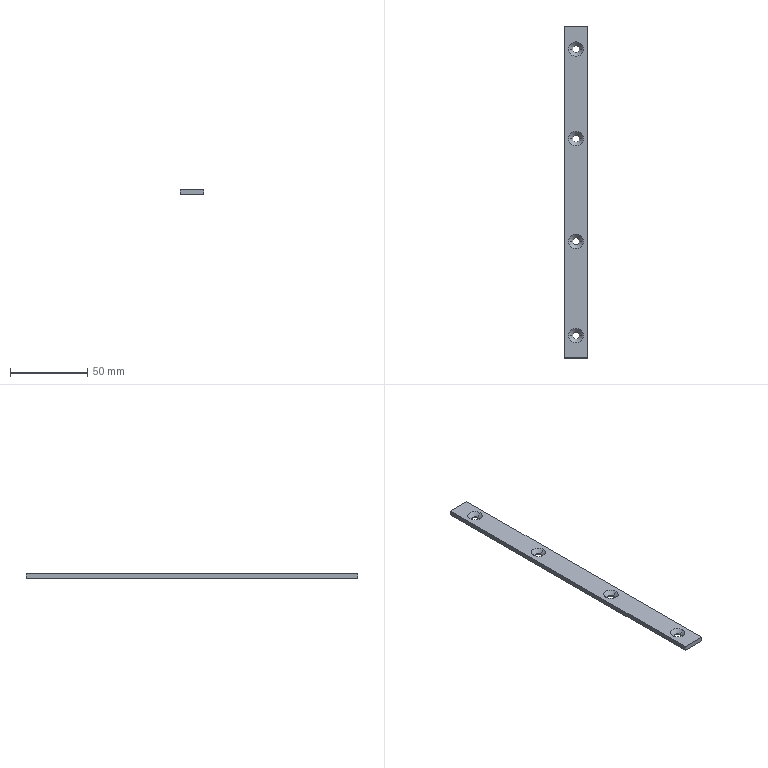Part | NX | features BREP 1 | 1 solid | 22 faces | box 15 x 215 x 3 mm | volume 9253 mm3 | cone 8 | cylinder 8 | plane 6 | commonest cylinder face diameters 4.5 x8
STEP:
#1=CARTESIAN_POINT('',(-4.7,-93.,3.));
#2=VERTEX_POINT('',#1);
#3=CARTESIAN_POINT('',(-2.25,-93.,0.55));
#4=VERTEX_POINT('',#3);
#5=CARTESIAN_POINT('',(-4.7,-93.,3.));
#6=DIRECTION('',(-0.7071,0.,0.7071));
#7=VECTOR('',#6,1000.);
#8=LINE('',#5,#7);
#9=EDGE_CURVE('',#2,#4,#8,.F.);
#10=ORIENTED_EDGE('',*,*,#9,.T.);
#11=CARTESIAN_POINT('',(2.25,-93.,0.55));
#12=VERTEX_POINT('',#11);
#13=CARTESIAN_POINT('',(0.,-93.,0.55));
#14=DIRECTION('',(0.,0.,1.));
#15=DIRECTION('',(1.,0.,0.));
#16=AXIS2_PLACEMENT_3D('',#13,#14,#15);
#17=CIRCLE('',#16,2.25);
#18=EDGE_CURVE('',#12,#4,#17,.T.);
#19=ORIENTED_EDGE('',*,*,#18,.F.);
#20=CARTESIAN_POINT('',(4.7,-93.,3.));
#21=VERTEX_POINT('',#20);
#22=CARTESIAN_POINT('',(4.7,-93.,3.));
#23=DIRECTION('',(0.7071,0.,0.7071));
#24=VECTOR('',#23,1000.);
#25=LINE('',#22,#24);
#26=EDGE_CURVE('',#21,#12,#25,.F.);
#27=ORIENTED_EDGE('',*,*,#26,.F.);
#28=CARTESIAN_POINT('',(0.,-93.,3.));
#29=DIRECTION('',(0.,0.,1.));
#30=DIRECTION('',(1.,0.,0.));
#31=AXIS2_PLACEMENT_3D('',#28,#29,#30);
#32=CIRCLE('',#31,4.7);
#33=EDGE_CURVE('',#21,#2,#32,.T.);
#34=ORIENTED_EDGE('',*,*,#33,.T.);
#35=EDGE_LOOP('',(#10,#19,#27,#34));
#36=FACE_BOUND('',#35,.T.);
#37=CARTESIAN_POINT('',(0.,-93.,3.));
#38=DIRECTION('',(0.,0.,1.));
#39=DIRECTION('',(1.,0.,0.));
#40=AXIS2_PLACEMENT_3D('',#37,#38,#39);
#41=CONICAL_SURFACE('',#40,4.7,0.7854);
#42=ADVANCED_FACE('',(#36),#41,.F.);
#43=CARTESIAN_POINT('',(-2.25,-93.,0.));
#44=VERTEX_POINT('',#43);
#45=CARTESIAN_POINT('',(-2.25,-93.,3.));
#46=DIRECTION('',(0.,0.,1.));
#47=VECTOR('',#46,1000.);
#48=LINE('',#45,#47);
#49=EDGE_CURVE('',#4,#44,#48,.F.);
#50=ORIENTED_EDGE('',*,*,#49,.T.);
#51=CARTESIAN_POINT('',(2.25,-93.,0.));
#52=VERTEX_POINT('',#51);
#53=CARTESIAN_POINT('',(0.,-93.,0.));
#54=DIRECTION('',(0.,0.,-1.));
#55=DIRECTION('',(-1.,0.,0.));
#56=AXIS2_PLACEMENT_3D('',#53,#54,#55);
#57=CIRCLE('',#56,2.25);
#58=EDGE_CURVE('',#44,#52,#57,.T.);
#59=ORIENTED_EDGE('',*,*,#58,.T.);
#60=CARTESIAN_POINT('',(2.25,-93.,3.));
#61=DIRECTION('',(0.,0.,1.));
#62=VECTOR('',#61,1000.);
#63=LINE('',#60,#62);
#64=EDGE_CURVE('',#12,#52,#63,.F.);
#65=ORIENTED_EDGE('',*,*,#64,.F.);
#66=ORIENTED_EDGE('',*,*,#18,.T.);
#67=EDGE_LOOP('',(#50,#59,#65,#66));
#68=FACE_BOUND('',#67,.T.);
#69=CARTESIAN_POINT('',(0.,-93.,3.));
#70=DIRECTION('',(0.,0.,1.));
#71=DIRECTION('',(1.,0.,0.));
#72=AXIS2_PLACEMENT_3D('',#69,#70,#71);
#73=CYLINDRICAL_SURFACE('',#72,2.25);
#74=ADVANCED_FACE('',(#68),#73,.F.);
#75=CARTESIAN_POINT('',(-4.7,-32.,3.));
#76=VERTEX_POINT('',#75);
#77=CARTESIAN_POINT('',(-2.25,-32.,0.55));
#78=VERTEX_POINT('',#77);
#79=CARTESIAN_POINT('',(-4.7,-32.,3.));
#80=DIRECTION('',(-0.7071,0.,0.7071));
#81=VECTOR('',#80,1000.);
#82=LINE('',#79,#81);
#83=EDGE_CURVE('',#76,#78,#82,.F.);
#84=ORIENTED_EDGE('',*,*,#83,.T.);
#85=CARTESIAN_POINT('',(2.25,-32.,0.55));
#86=VERTEX_POINT('',#85);
#87=CARTESIAN_POINT('',(0.,-32.,0.55));
#88=DIRECTION('',(0.,0.,1.));
#89=DIRECTION('',(1.,0.,0.));
#90=AXIS2_PLACEMENT_3D('',#87,#88,#89);
#91=CIRCLE('',#90,2.25);
#92=EDGE_CURVE('',#86,#78,#91,.T.);
#93=ORIENTED_EDGE('',*,*,#92,.F.);
#94=CARTESIAN_POINT('',(4.7,-32.,3.));
#95=VERTEX_POINT('',#94);
#96=CARTESIAN_POINT('',(4.7,-32.,3.));
#97=DIRECTION('',(0.7071,0.,0.7071));
#98=VECTOR('',#97,1000.);
#99=LINE('',#96,#98);
#100=EDGE_CURVE('',#95,#86,#99,.F.);
#101=ORIENTED_EDGE('',*,*,#100,.F.);
#102=CARTESIAN_POINT('',(0.,-32.,3.));
#103=DIRECTION('',(0.,0.,1.));
#104=DIRECTION('',(1.,0.,0.));
#105=AXIS2_PLACEMENT_3D('',#102,#103,#104);
#106=CIRCLE('',#105,4.7);
#107=EDGE_CURVE('',#95,#76,#106,.T.);
#108=ORIENTED_EDGE('',*,*,#107,.T.);
#109=EDGE_LOOP('',(#84,#93,#101,#108));
#110=FACE_BOUND('',#109,.T.);
#111=CARTESIAN_POINT('',(0.,-32.,3.));
#112=DIRECTION('',(0.,0.,1.));
#113=DIRECTION('',(1.,0.,0.));
#114=AXIS2_PLACEMENT_3D('',#111,#112,#113);
#115=CONICAL_SURFACE('',#114,4.7,0.7854);
#116=ADVANCED_FACE('',(#110),#115,.F.);
#117=CARTESIAN_POINT('',(-2.25,-32.,0.));
#118=VERTEX_POINT('',#117);
#119=CARTESIAN_POINT('',(-2.25,-32.,3.));
#120=DIRECTION('',(0.,0.,1.));
#121=VECTOR('',#120,1000.);
#122=LINE('',#119,#121);
#123=EDGE_CURVE('',#78,#118,#122,.F.);
#124=ORIENTED_EDGE('',*,*,#123,.T.);
#125=CARTESIAN_POINT('',(2.25,-32.,0.));
#126=VERTEX_POINT('',#125);
#127=CARTESIAN_POINT('',(0.,-32.,0.));
#128=DIRECTION('',(0.,0.,-1.));
#129=DIRECTION('',(-1.,0.,0.));
#130=AXIS2_PLACEMENT_3D('',#127,#128,#129);
#131=CIRCLE('',#130,2.25);
#132=EDGE_CURVE('',#118,#126,#131,.T.);
#133=ORIENTED_EDGE('',*,*,#132,.T.);
#134=CARTESIAN_POINT('',(2.25,-32.,3.));
#135=DIRECTION('',(0.,0.,1.));
#136=VECTOR('',#135,1000.);
#137=LINE('',#134,#136);
#138=EDGE_CURVE('',#86,#126,#137,.F.);
#139=ORIENTED_EDGE('',*,*,#138,.F.);
#140=ORIENTED_EDGE('',*,*,#92,.T.);
#141=EDGE_LOOP('',(#124,#133,#139,#140));
#142=FACE_BOUND('',#141,.T.);
#143=CARTESIAN_POINT('',(0.,-32.,3.));
#144=DIRECTION('',(0.,0.,1.));
#145=DIRECTION('',(1.,0.,0.));
#146=AXIS2_PLACEMENT_3D('',#143,#144,#145);
#147=CYLINDRICAL_SURFACE('',#146,2.25);
#148=ADVANCED_FACE('',(#142),#147,.F.);
#149=CARTESIAN_POINT('',(-4.7,34.5,3.));
#150=VERTEX_POINT('',#149);
#151=CARTESIAN_POINT('',(-2.25,34.5,0.55));
#152=VERTEX_POINT('',#151);
#153=CARTESIAN_POINT('',(-4.7,34.5,3.));
#154=DIRECTION('',(-0.7071,0.,0.7071));
#155=VECTOR('',#154,1000.);
#156=LINE('',#153,#155);
#157=EDGE_CURVE('',#150,#152,#156,.F.);
#158=ORIENTED_EDGE('',*,*,#157,.T.);
#159=CARTESIAN_POINT('',(2.25,34.5,0.55));
#160=VERTEX_POINT('',#159);
#161=CARTESIAN_POINT('',(0.,34.5,0.55));
#162=DIRECTION('',(0.,0.,1.));
#163=DIRECTION('',(1.,0.,0.));
#164=AXIS2_PLACEMENT_3D('',#161,#162,#163);
#165=CIRCLE('',#164,2.25);
#166=EDGE_CURVE('',#160,#152,#165,.T.);
#167=ORIENTED_EDGE('',*,*,#166,.F.);
#168=CARTESIAN_POINT('',(4.7,34.5,3.));
#169=VERTEX_POINT('',#168);
#170=CARTESIAN_POINT('',(4.7,34.5,3.));
#171=DIRECTION('',(0.7071,0.,0.7071));
#172=VECTOR('',#171,1000.);
#173=LINE('',#170,#172);
#174=EDGE_CURVE('',#169,#160,#173,.F.);
#175=ORIENTED_EDGE('',*,*,#174,.F.);
#176=CARTESIAN_POINT('',(0.,34.5,3.));
#177=DIRECTION('',(0.,0.,1.));
#178=DIRECTION('',(1.,0.,0.));
#179=AXIS2_PLACEMENT_3D('',#176,#177,#178);
#180=CIRCLE('',#179,4.7);
#181=EDGE_CURVE('',#169,#150,#180,.T.);
#182=ORIENTED_EDGE('',*,*,#181,.T.);
#183=EDGE_LOOP('',(#158,#167,#175,#182));
#184=FACE_BOUND('',#183,.T.);
#185=CARTESIAN_POINT('',(0.,34.5,3.));
#186=DIRECTION('',(0.,0.,1.));
#187=DIRECTION('',(1.,0.,0.));
#188=AXIS2_PLACEMENT_3D('',#185,#186,#187);
#189=CONICAL_SURFACE('',#188,4.7,0.7854);
#190=ADVANCED_FACE('',(#184),#189,.F.);
#191=CARTESIAN_POINT('',(-2.25,34.5,0.));
#192=VERTEX_POINT('',#191);
#193=CARTESIAN_POINT('',(-2.25,34.5,3.));
#194=DIRECTION('',(0.,0.,1.));
#195=VECTOR('',#194,1000.);
#196=LINE('',#193,#195);
#197=EDGE_CURVE('',#152,#192,#196,.F.);
#198=ORIENTED_EDGE('',*,*,#197,.T.);
#199=CARTESIAN_POINT('',(2.25,34.5,0.));
#200=VERTEX_POINT('',#199);
#201=CARTESIAN_POINT('',(0.,34.5,0.));
#202=DIRECTION('',(0.,0.,-1.));
#203=DIRECTION('',(-1.,0.,0.));
#204=AXIS2_PLACEMENT_3D('',#201,#202,#203);
#205=CIRCLE('',#204,2.25);
#206=EDGE_CURVE('',#192,#200,#205,.T.);
#207=ORIENTED_EDGE('',*,*,#206,.T.);
#208=CARTESIAN_POINT('',(2.25,34.5,3.));
#209=DIRECTION('',(0.,0.,1.));
#210=VECTOR('',#209,1000.);
#211=LINE('',#208,#210);
#212=EDGE_CURVE('',#160,#200,#211,.F.);
#213=ORIENTED_EDGE('',*,*,#212,.F.);
#214=ORIENTED_EDGE('',*,*,#166,.T.);
#215=EDGE_LOOP('',(#198,#207,#213,#214));
#216=FACE_BOUND('',#215,.T.);
#217=CARTESIAN_POINT('',(0.,34.5,3.));
#218=DIRECTION('',(0.,0.,1.));
#219=DIRECTION('',(1.,0.,0.));
#220=AXIS2_PLACEMENT_3D('',#217,#218,#219);
#221=CYLINDRICAL_SURFACE('',#220,2.25);
#222=ADVANCED_FACE('',(#216),#221,.F.);
#223=CARTESIAN_POINT('',(-4.7,92.5,3.));
#224=VERTEX_POINT('',#223);
#225=CARTESIAN_POINT('',(-2.25,92.5,0.55));
#226=VERTEX_POINT('',#225);
#227=CARTESIAN_POINT('',(-4.7,92.5,3.));
#228=DIRECTION('',(-0.7071,0.,0.7071));
#229=VECTOR('',#228,1000.);
#230=LINE('',#227,#229);
#231=EDGE_CURVE('',#224,#226,#230,.F.);
#232=ORIENTED_EDGE('',*,*,#231,.T.);
#233=CARTESIAN_POINT('',(2.25,92.5,0.55));
#234=VERTEX_POINT('',#233);
#235=CARTESIAN_POINT('',(0.,92.5,0.55));
#236=DIRECTION('',(0.,0.,1.));
#237=DIRECTION('',(1.,0.,0.));
#238=AXIS2_PLACEMENT_3D('',#235,#236,#237);
#239=CIRCLE('',#238,2.25);
#240=EDGE_CURVE('',#234,#226,#239,.T.);
#241=ORIENTED_EDGE('',*,*,#240,.F.);
#242=CARTESIAN_POINT('',(4.7,92.5,3.));
#243=VERTEX_POINT('',#242);
#244=CARTESIAN_POINT('',(4.7,92.5,3.));
#245=DIRECTION('',(0.7071,0.,0.7071));
#246=VECTOR('',#245,1000.);
#247=LINE('',#244,#246);
#248=EDGE_CURVE('',#243,#234,#247,.F.);
#249=ORIENTED_EDGE('',*,*,#248,.F.);
#250=CARTESIAN_POINT('',(0.,92.5,3.));
#251=DIRECTION('',(0.,0.,1.));
#252=DIRECTION('',(1.,0.,0.));
#253=AXIS2_PLACEMENT_3D('',#250,#251,#252);
#254=CIRCLE('',#253,4.7);
#255=EDGE_CURVE('',#243,#224,#254,.T.);
#256=ORIENTED_EDGE('',*,*,#255,.T.);
#257=EDGE_LOOP('',(#232,#241,#249,#256));
#258=FACE_BOUND('',#257,.T.);
#259=CARTESIAN_POINT('',(0.,92.5,3.));
#260=DIRECTION('',(0.,0.,1.));
#261=DIRECTION('',(1.,0.,0.));
#262=AXIS2_PLACEMENT_3D('',#259,#260,#261);
#263=CONICAL_SURFACE('',#262,4.7,0.7854);
#264=ADVANCED_FACE('',(#258),#263,.F.);
#265=CARTESIAN_POINT('',(-2.25,92.5,0.));
#266=VERTEX_POINT('',#265);
#267=CARTESIAN_POINT('',(-2.25,92.5,3.));
#268=DIRECTION('',(0.,0.,1.));
#269=VECTOR('',#268,1000.);
#270=LINE('',#267,#269);
#271=EDGE_CURVE('',#226,#266,#270,.F.);
#272=ORIENTED_EDGE('',*,*,#271,.T.);
#273=CARTESIAN_POINT('',(2.25,92.5,0.));
#274=VERTEX_POINT('',#273);
#275=CARTESIAN_POINT('',(0.,92.5,0.));
#276=DIRECTION('',(0.,0.,-1.));
#277=DIRECTION('',(-1.,0.,0.));
#278=AXIS2_PLACEMENT_3D('',#275,#276,#277);
#279=CIRCLE('',#278,2.25);
#280=EDGE_CURVE('',#266,#274,#279,.T.);
#281=ORIENTED_EDGE('',*,*,#280,.T.);
#282=CARTESIAN_POINT('',(2.25,92.5,3.));
#283=DIRECTION('',(0.,0.,1.));
#284=VECTOR('',#283,1000.);
#285=LINE('',#282,#284);
#286=EDGE_CURVE('',#234,#274,#285,.F.);
#287=ORIENTED_EDGE('',*,*,#286,.F.);
#288=ORIENTED_EDGE('',*,*,#240,.T.);
#289=EDGE_LOOP('',(#272,#281,#287,#288));
#290=FACE_BOUND('',#289,.T.);
#291=CARTESIAN_POINT('',(0.,92.5,3.));
#292=DIRECTION('',(0.,0.,1.));
#293=DIRECTION('',(1.,0.,0.));
#294=AXIS2_PLACEMENT_3D('',#291,#292,#293);
#295=CYLINDRICAL_SURFACE('',#294,2.25);
#296=ADVANCED_FACE('',(#290),#295,.F.);
#297=CARTESIAN_POINT('',(7.5,-107.5,0.));
#298=VERTEX_POINT('',#297);
#299=CARTESIAN_POINT('',(7.5,107.5,0.));
#300=VERTEX_POINT('',#299);
#301=CARTESIAN_POINT('',(7.5,-107.5,0.));
#302=DIRECTION('',(0.,1.,0.));
#303=VECTOR('',#302,1000.);
#304=LINE('',#301,#303);
#305=EDGE_CURVE('',#298,#300,#304,.T.);
#306=ORIENTED_EDGE('',*,*,#305,.F.);
#307=CARTESIAN_POINT('',(-7.5,-107.5,0.));
#308=VERTEX_POINT('',#307);
#309=CARTESIAN_POINT('',(-7.5,-107.5,0.));
#310=DIRECTION('',(1.,0.,0.));
#311=VECTOR('',#310,1000.);
#312=LINE('',#309,#311);
#313=EDGE_CURVE('',#308,#298,#312,.T.);
#314=ORIENTED_EDGE('',*,*,#313,.F.);
#315=CARTESIAN_POINT('',(-7.5,107.5,0.));
#316=VERTEX_POINT('',#315);
#317=CARTESIAN_POINT('',(-7.5,-107.5,0.));
#318=DIRECTION('',(0.,-1.,0.));
#319=VECTOR('',#318,1000.);
#320=LINE('',#317,#319);
#321=EDGE_CURVE('',#316,#308,#320,.T.);
#322=ORIENTED_EDGE('',*,*,#321,.F.);
#323=CARTESIAN_POINT('',(-7.5,107.5,0.));
#324=DIRECTION('',(-1.,0.,0.));
#325=VECTOR('',#324,1000.);
#326=LINE('',#323,#325);
#327=EDGE_CURVE('',#300,#316,#326,.T.);
#328=ORIENTED_EDGE('',*,*,#327,.F.);
#329=EDGE_LOOP('',(#306,#314,#322,#328));
#330=FACE_BOUND('',#329,.T.);
#331=CARTESIAN_POINT('',(0.,92.5,0.));
#332=DIRECTION('',(0.,0.,-1.));
#333=DIRECTION('',(-1.,0.,0.));
#334=AXIS2_PLACEMENT_3D('',#331,#332,#333);
#335=CIRCLE('',#334,2.25);
#336=EDGE_CURVE('',#274,#266,#335,.T.);
#337=ORIENTED_EDGE('',*,*,#336,.F.);
#338=ORIENTED_EDGE('',*,*,#280,.F.);
#339=EDGE_LOOP('',(#337,#338));
#340=FACE_BOUND('',#339,.T.);
#341=CARTESIAN_POINT('',(0.,34.5,0.));
#342=DIRECTION('',(0.,0.,-1.));
#343=DIRECTION('',(-1.,0.,0.));
#344=AXIS2_PLACEMENT_3D('',#341,#342,#343);
#345=CIRCLE('',#344,2.25);
#346=EDGE_CURVE('',#200,#192,#345,.T.);
#347=ORIENTED_EDGE('',*,*,#346,.F.);
#348=ORIENTED_EDGE('',*,*,#206,.F.);
#349=EDGE_LOOP('',(#347,#348));
#350=FACE_BOUND('',#349,.T.);
#351=CARTESIAN_POINT('',(0.,-32.,0.));
#352=DIRECTION('',(0.,0.,-1.));
#353=DIRECTION('',(-1.,0.,0.));
#354=AXIS2_PLACEMENT_3D('',#351,#352,#353);
#355=CIRCLE('',#354,2.25);
#356=EDGE_CURVE('',#126,#118,#355,.T.);
#357=ORIENTED_EDGE('',*,*,#356,.F.);
#358=ORIENTED_EDGE('',*,*,#132,.F.);
#359=EDGE_LOOP('',(#357,#358));
#360=FACE_BOUND('',#359,.T.);
#361=CARTESIAN_POINT('',(0.,-93.,0.));
#362=DIRECTION('',(0.,0.,-1.));
#363=DIRECTION('',(-1.,0.,0.));
#364=AXIS2_PLACEMENT_3D('',#361,#362,#363);
#365=CIRCLE('',#364,2.25);
#366=EDGE_CURVE('',#52,#44,#365,.T.);
#367=ORIENTED_EDGE('',*,*,#366,.F.);
#368=ORIENTED_EDGE('',*,*,#58,.F.);
#369=EDGE_LOOP('',(#367,#368));
#370=FACE_BOUND('',#369,.T.);
#371=CARTESIAN_POINT('',(0.,0.,0.));
#372=DIRECTION('',(0.,0.,-1.));
#373=DIRECTION('',(-1.,0.,0.));
#374=AXIS2_PLACEMENT_3D('',#371,#372,#373);
#375=PLANE('',#374);
#376=ADVANCED_FACE('',(#330,#340,#350,#360,#370),#375,.T.);
#377=CARTESIAN_POINT('',(7.5,-107.5,3.));
#378=VERTEX_POINT('',#377);
#379=CARTESIAN_POINT('',(7.5,107.5,3.));
#380=VERTEX_POINT('',#379);
#381=CARTESIAN_POINT('',(7.5,-107.5,3.));
#382=DIRECTION('',(0.,1.,0.));
#383=VECTOR('',#382,1000.);
#384=LINE('',#381,#383);
#385=EDGE_CURVE('',#378,#380,#384,.T.);
#386=ORIENTED_EDGE('',*,*,#385,.T.);
#387=CARTESIAN_POINT('',(-7.5,107.5,3.));
#388=VERTEX_POINT('',#387);
#389=CARTESIAN_POINT('',(-7.5,107.5,3.));
#390=DIRECTION('',(-1.,0.,0.));
#391=VECTOR('',#390,1000.);
#392=LINE('',#389,#391);
#393=EDGE_CURVE('',#380,#388,#392,.T.);
#394=ORIENTED_EDGE('',*,*,#393,.T.);
#395=CARTESIAN_POINT('',(-7.5,-107.5,3.));
#396=VERTEX_POINT('',#395);
#397=CARTESIAN_POINT('',(-7.5,-107.5,3.));
#398=DIRECTION('',(0.,-1.,0.));
#399=VECTOR('',#398,1000.);
#400=LINE('',#397,#399);
#401=EDGE_CURVE('',#388,#396,#400,.T.);
#402=ORIENTED_EDGE('',*,*,#401,.T.);
#403=CARTESIAN_POINT('',(-7.5,-107.5,3.));
#404=DIRECTION('',(1.,0.,0.));
#405=VECTOR('',#404,1000.);
#406=LINE('',#403,#405);
#407=EDGE_CURVE('',#396,#378,#406,.T.);
#408=ORIENTED_EDGE('',*,*,#407,.T.);
#409=EDGE_LOOP('',(#386,#394,#402,#408));
#410=FACE_BOUND('',#409,.T.);
#411=ORIENTED_EDGE('',*,*,#255,.F.);
#412=CARTESIAN_POINT('',(0.,92.5,3.));
#413=DIRECTION('',(0.,0.,1.));
#414=DIRECTION('',(1.,0.,0.));
#415=AXIS2_PLACEMENT_3D('',#412,#413,#414);
#416=CIRCLE('',#415,4.7);
#417=EDGE_CURVE('',#224,#243,#416,.T.);
#418=ORIENTED_EDGE('',*,*,#417,.F.);
#419=EDGE_LOOP('',(#411,#418));
#420=FACE_BOUND('',#419,.T.);
#421=ORIENTED_EDGE('',*,*,#181,.F.);
#422=CARTESIAN_POINT('',(0.,34.5,3.));
#423=DIRECTION('',(0.,0.,1.));
#424=DIRECTION('',(1.,0.,0.));
#425=AXIS2_PLACEMENT_3D('',#422,#423,#424);
#426=CIRCLE('',#425,4.7);
#427=EDGE_CURVE('',#150,#169,#426,.T.);
#428=ORIENTED_EDGE('',*,*,#427,.F.);
#429=EDGE_LOOP('',(#421,#428));
#430=FACE_BOUND('',#429,.T.);
#431=ORIENTED_EDGE('',*,*,#107,.F.);
#432=CARTESIAN_POINT('',(0.,-32.,3.));
#433=DIRECTION('',(0.,0.,1.));
#434=DIRECTION('',(1.,0.,0.));
#435=AXIS2_PLACEMENT_3D('',#432,#433,#434);
#436=CIRCLE('',#435,4.7);
#437=EDGE_CURVE('',#76,#95,#436,.T.);
#438=ORIENTED_EDGE('',*,*,#437,.F.);
#439=EDGE_LOOP('',(#431,#438));
#440=FACE_BOUND('',#439,.T.);
#441=ORIENTED_EDGE('',*,*,#33,.F.);
#442=CARTESIAN_POINT('',(0.,-93.,3.));
#443=DIRECTION('',(0.,0.,1.));
#444=DIRECTION('',(1.,0.,0.));
#445=AXIS2_PLACEMENT_3D('',#442,#443,#444);
#446=CIRCLE('',#445,4.7);
#447=EDGE_CURVE('',#2,#21,#446,.T.);
#448=ORIENTED_EDGE('',*,*,#447,.F.);
#449=EDGE_LOOP('',(#441,#448));
#450=FACE_BOUND('',#449,.T.);
#451=CARTESIAN_POINT('',(0.,0.,3.));
#452=DIRECTION('',(0.,0.,-1.));
#453=DIRECTION('',(-1.,0.,0.));
#454=AXIS2_PLACEMENT_3D('',#451,#452,#453);
#455=PLANE('',#454);
#456=ADVANCED_FACE('',(#410,#420,#430,#440,#450),#455,.F.);
#457=ORIENTED_EDGE('',*,*,#313,.T.);
#458=CARTESIAN_POINT('',(7.5,-107.5,3.));
#459=DIRECTION('',(0.,0.,-1.));
#460=VECTOR('',#459,1000.);
#461=LINE('',#458,#460);
#462=EDGE_CURVE('',#378,#298,#461,.T.);
#463=ORIENTED_EDGE('',*,*,#462,.F.);
#464=ORIENTED_EDGE('',*,*,#407,.F.);
#465=CARTESIAN_POINT('',(-7.5,-107.5,3.));
#466=DIRECTION('',(0.,0.,-1.));
#467=VECTOR('',#466,1000.);
#468=LINE('',#465,#467);
#469=EDGE_CURVE('',#396,#308,#468,.T.);
#470=ORIENTED_EDGE('',*,*,#469,.T.);
#471=EDGE_LOOP('',(#457,#463,#464,#470));
#472=FACE_BOUND('',#471,.T.);
#473=CARTESIAN_POINT('',(-7.5,-107.5,3.));
#474=DIRECTION('',(0.,1.,0.));
#475=DIRECTION('',(0.,0.,1.));
#476=AXIS2_PLACEMENT_3D('',#473,#474,#475);
#477=PLANE('',#476);
#478=ADVANCED_FACE('',(#472),#477,.F.);
#479=ORIENTED_EDGE('',*,*,#321,.T.);
#480=ORIENTED_EDGE('',*,*,#469,.F.);
#481=ORIENTED_EDGE('',*,*,#401,.F.);
#482=CARTESIAN_POINT('',(-7.5,107.5,3.));
#483=DIRECTION('',(0.,0.,-1.));
#484=VECTOR('',#483,1000.);
#485=LINE('',#482,#484);
#486=EDGE_CURVE('',#388,#316,#485,.T.);
#487=ORIENTED_EDGE('',*,*,#486,.T.);
#488=EDGE_LOOP('',(#479,#480,#481,#487));
#489=FACE_BOUND('',#488,.T.);
#490=CARTESIAN_POINT('',(-7.5,-107.5,3.));
#491=DIRECTION('',(1.,0.,0.));
#492=DIRECTION('',(0.,0.,-1.));
#493=AXIS2_PLACEMENT_3D('',#490,#491,#492);
#494=PLANE('',#493);
#495=ADVANCED_FACE('',(#489),#494,.F.);
#496=ORIENTED_EDGE('',*,*,#327,.T.);
#497=ORIENTED_EDGE('',*,*,#486,.F.);
#498=ORIENTED_EDGE('',*,*,#393,.F.);
#499=CARTESIAN_POINT('',(7.5,107.5,3.));
#500=DIRECTION('',(0.,0.,-1.));
#501=VECTOR('',#500,1000.);
#502=LINE('',#499,#501);
#503=EDGE_CURVE('',#380,#300,#502,.T.);
#504=ORIENTED_EDGE('',*,*,#503,.T.);
#505=EDGE_LOOP('',(#496,#497,#498,#504));
#506=FACE_BOUND('',#505,.T.);
#507=CARTESIAN_POINT('',(-7.5,107.5,3.));
#508=DIRECTION('',(0.,-1.,0.));
#509=DIRECTION('',(0.,0.,-1.));
#510=AXIS2_PLACEMENT_3D('',#507,#508,#509);
#511=PLANE('',#510);
#512=ADVANCED_FACE('',(#506),#511,.F.);
#513=ORIENTED_EDGE('',*,*,#305,.T.);
#514=ORIENTED_EDGE('',*,*,#503,.F.);
#515=ORIENTED_EDGE('',*,*,#385,.F.);
#516=ORIENTED_EDGE('',*,*,#462,.T.);
#517=EDGE_LOOP('',(#513,#514,#515,#516));
#518=FACE_BOUND('',#517,.T.);
#519=CARTESIAN_POINT('',(7.5,-107.5,3.));
#520=DIRECTION('',(-1.,0.,0.));
#521=DIRECTION('',(0.,0.,1.));
#522=AXIS2_PLACEMENT_3D('',#519,#520,#521);
#523=PLANE('',#522);
#524=ADVANCED_FACE('',(#518),#523,.F.);
#525=ORIENTED_EDGE('',*,*,#336,.T.);
#526=ORIENTED_EDGE('',*,*,#271,.F.);
#527=CARTESIAN_POINT('',(0.,92.5,0.55));
#528=DIRECTION('',(0.,0.,1.));
#529=DIRECTION('',(1.,0.,0.));
#530=AXIS2_PLACEMENT_3D('',#527,#528,#529);
#531=CIRCLE('',#530,2.25);
#532=EDGE_CURVE('',#226,#234,#531,.T.);
#533=ORIENTED_EDGE('',*,*,#532,.T.);
#534=ORIENTED_EDGE('',*,*,#286,.T.);
#535=EDGE_LOOP('',(#525,#526,#533,#534));
#536=FACE_BOUND('',#535,.T.);
#537=CARTESIAN_POINT('',(0.,92.5,3.));
#538=DIRECTION('',(0.,0.,1.));
#539=DIRECTION('',(1.,0.,0.));
#540=AXIS2_PLACEMENT_3D('',#537,#538,#539);
#541=CYLINDRICAL_SURFACE('',#540,2.25);
#542=ADVANCED_FACE('',(#536),#541,.F.);
#543=ORIENTED_EDGE('',*,*,#532,.F.);
#544=ORIENTED_EDGE('',*,*,#231,.F.);
#545=ORIENTED_EDGE('',*,*,#417,.T.);
#546=ORIENTED_EDGE('',*,*,#248,.T.);
#547=EDGE_LOOP('',(#543,#544,#545,#546));
#548=FACE_BOUND('',#547,.T.);
#549=CARTESIAN_POINT('',(0.,92.5,3.));
#550=DIRECTION('',(0.,0.,1.));
#551=DIRECTION('',(1.,0.,0.));
#552=AXIS2_PLACEMENT_3D('',#549,#550,#551);
#553=CONICAL_SURFACE('',#552,4.7,0.7854);
#554=ADVANCED_FACE('',(#548),#553,.F.);
#555=ORIENTED_EDGE('',*,*,#346,.T.);
#556=ORIENTED_EDGE('',*,*,#197,.F.);
#557=CARTESIAN_POINT('',(0.,34.5,0.55));
#558=DIRECTION('',(0.,0.,1.));
#559=DIRECTION('',(1.,0.,0.));
#560=AXIS2_PLACEMENT_3D('',#557,#558,#559);
#561=CIRCLE('',#560,2.25);
#562=EDGE_CURVE('',#152,#160,#561,.T.);
#563=ORIENTED_EDGE('',*,*,#562,.T.);
#564=ORIENTED_EDGE('',*,*,#212,.T.);
#565=EDGE_LOOP('',(#555,#556,#563,#564));
#566=FACE_BOUND('',#565,.T.);
#567=CARTESIAN_POINT('',(0.,34.5,3.));
#568=DIRECTION('',(0.,0.,1.));
#569=DIRECTION('',(1.,0.,0.));
#570=AXIS2_PLACEMENT_3D('',#567,#568,#569);
#571=CYLINDRICAL_SURFACE('',#570,2.25);
#572=ADVANCED_FACE('',(#566),#571,.F.);
#573=ORIENTED_EDGE('',*,*,#562,.F.);
#574=ORIENTED_EDGE('',*,*,#157,.F.);
#575=ORIENTED_EDGE('',*,*,#427,.T.);
#576=ORIENTED_EDGE('',*,*,#174,.T.);
#577=EDGE_LOOP('',(#573,#574,#575,#576));
#578=FACE_BOUND('',#577,.T.);
#579=CARTESIAN_POINT('',(0.,34.5,3.));
#580=DIRECTION('',(0.,0.,1.));
#581=DIRECTION('',(1.,0.,0.));
#582=AXIS2_PLACEMENT_3D('',#579,#580,#581);
#583=CONICAL_SURFACE('',#582,4.7,0.7854);
#584=ADVANCED_FACE('',(#578),#583,.F.);
#585=ORIENTED_EDGE('',*,*,#356,.T.);
#586=ORIENTED_EDGE('',*,*,#123,.F.);
#587=CARTESIAN_POINT('',(0.,-32.,0.55));
#588=DIRECTION('',(0.,0.,1.));
#589=DIRECTION('',(1.,0.,0.));
#590=AXIS2_PLACEMENT_3D('',#587,#588,#589);
#591=CIRCLE('',#590,2.25);
#592=EDGE_CURVE('',#78,#86,#591,.T.);
#593=ORIENTED_EDGE('',*,*,#592,.T.);
#594=ORIENTED_EDGE('',*,*,#138,.T.);
#595=EDGE_LOOP('',(#585,#586,#593,#594));
#596=FACE_BOUND('',#595,.T.);
#597=CARTESIAN_POINT('',(0.,-32.,3.));
#598=DIRECTION('',(0.,0.,1.));
#599=DIRECTION('',(1.,0.,0.));
#600=AXIS2_PLACEMENT_3D('',#597,#598,#599);
#601=CYLINDRICAL_SURFACE('',#600,2.25);
#602=ADVANCED_FACE('',(#596),#601,.F.);
#603=ORIENTED_EDGE('',*,*,#592,.F.);
#604=ORIENTED_EDGE('',*,*,#83,.F.);
#605=ORIENTED_EDGE('',*,*,#437,.T.);
#606=ORIENTED_EDGE('',*,*,#100,.T.);
#607=EDGE_LOOP('',(#603,#604,#605,#606));
#608=FACE_BOUND('',#607,.T.);
#609=CARTESIAN_POINT('',(0.,-32.,3.));
#610=DIRECTION('',(0.,0.,1.));
#611=DIRECTION('',(1.,0.,0.));
#612=AXIS2_PLACEMENT_3D('',#609,#610,#611);
#613=CONICAL_SURFACE('',#612,4.7,0.7854);
#614=ADVANCED_FACE('',(#608),#613,.F.);
#615=ORIENTED_EDGE('',*,*,#366,.T.);
#616=ORIENTED_EDGE('',*,*,#49,.F.);
#617=CARTESIAN_POINT('',(0.,-93.,0.55));
#618=DIRECTION('',(0.,0.,1.));
#619=DIRECTION('',(1.,0.,0.));
#620=AXIS2_PLACEMENT_3D('',#617,#618,#619);
#621=CIRCLE('',#620,2.25);
#622=EDGE_CURVE('',#4,#12,#621,.T.);
#623=ORIENTED_EDGE('',*,*,#622,.T.);
#624=ORIENTED_EDGE('',*,*,#64,.T.);
#625=EDGE_LOOP('',(#615,#616,#623,#624));
#626=FACE_BOUND('',#625,.T.);
#627=CARTESIAN_POINT('',(0.,-93.,3.));
#628=DIRECTION('',(0.,0.,1.));
#629=DIRECTION('',(1.,0.,0.));
#630=AXIS2_PLACEMENT_3D('',#627,#628,#629);
#631=CYLINDRICAL_SURFACE('',#630,2.25);
#632=ADVANCED_FACE('',(#626),#631,.F.);
#633=ORIENTED_EDGE('',*,*,#622,.F.);
#634=ORIENTED_EDGE('',*,*,#9,.F.);
#635=ORIENTED_EDGE('',*,*,#447,.T.);
#636=ORIENTED_EDGE('',*,*,#26,.T.);
#637=EDGE_LOOP('',(#633,#634,#635,#636));
#638=FACE_BOUND('',#637,.T.);
#639=CARTESIAN_POINT('',(0.,-93.,3.));
#640=DIRECTION('',(0.,0.,1.));
#641=DIRECTION('',(1.,0.,0.));
#642=AXIS2_PLACEMENT_3D('',#639,#640,#641);
#643=CONICAL_SURFACE('',#642,4.7,0.7854);
#644=ADVANCED_FACE('',(#638),#643,.F.);
#645=CLOSED_SHELL('',(#42,#74,#116,#148,#190,#222,#264,#296,#376,#456,#478,#495,#512,#524,#542,#554,#572,#584,#602,#614,#632,#644));
#646=MANIFOLD_SOLID_BREP('',#645);
#647=(LENGTH_UNIT()NAMED_UNIT(*)SI_UNIT(.MILLI.,.METRE.));
#648=UNCERTAINTY_MEASURE_WITH_UNIT(LENGTH_MEASURE(0.00001),#647,'','');
#649=(NAMED_UNIT(*)PLANE_ANGLE_UNIT()SI_UNIT($,.RADIAN.));
#650=(NAMED_UNIT(*)SI_UNIT($,.STERADIAN.)SOLID_ANGLE_UNIT());
#651=(GEOMETRIC_REPRESENTATION_CONTEXT(3)GLOBAL_UNCERTAINTY_ASSIGNED_CONTEXT((#648))GLOBAL_UNIT_ASSIGNED_CONTEXT((#647,#649,#650))REPRESENTATION_CONTEXT('',''));
#652=ADVANCED_BREP_SHAPE_REPRESENTATION('',(#646),#651);